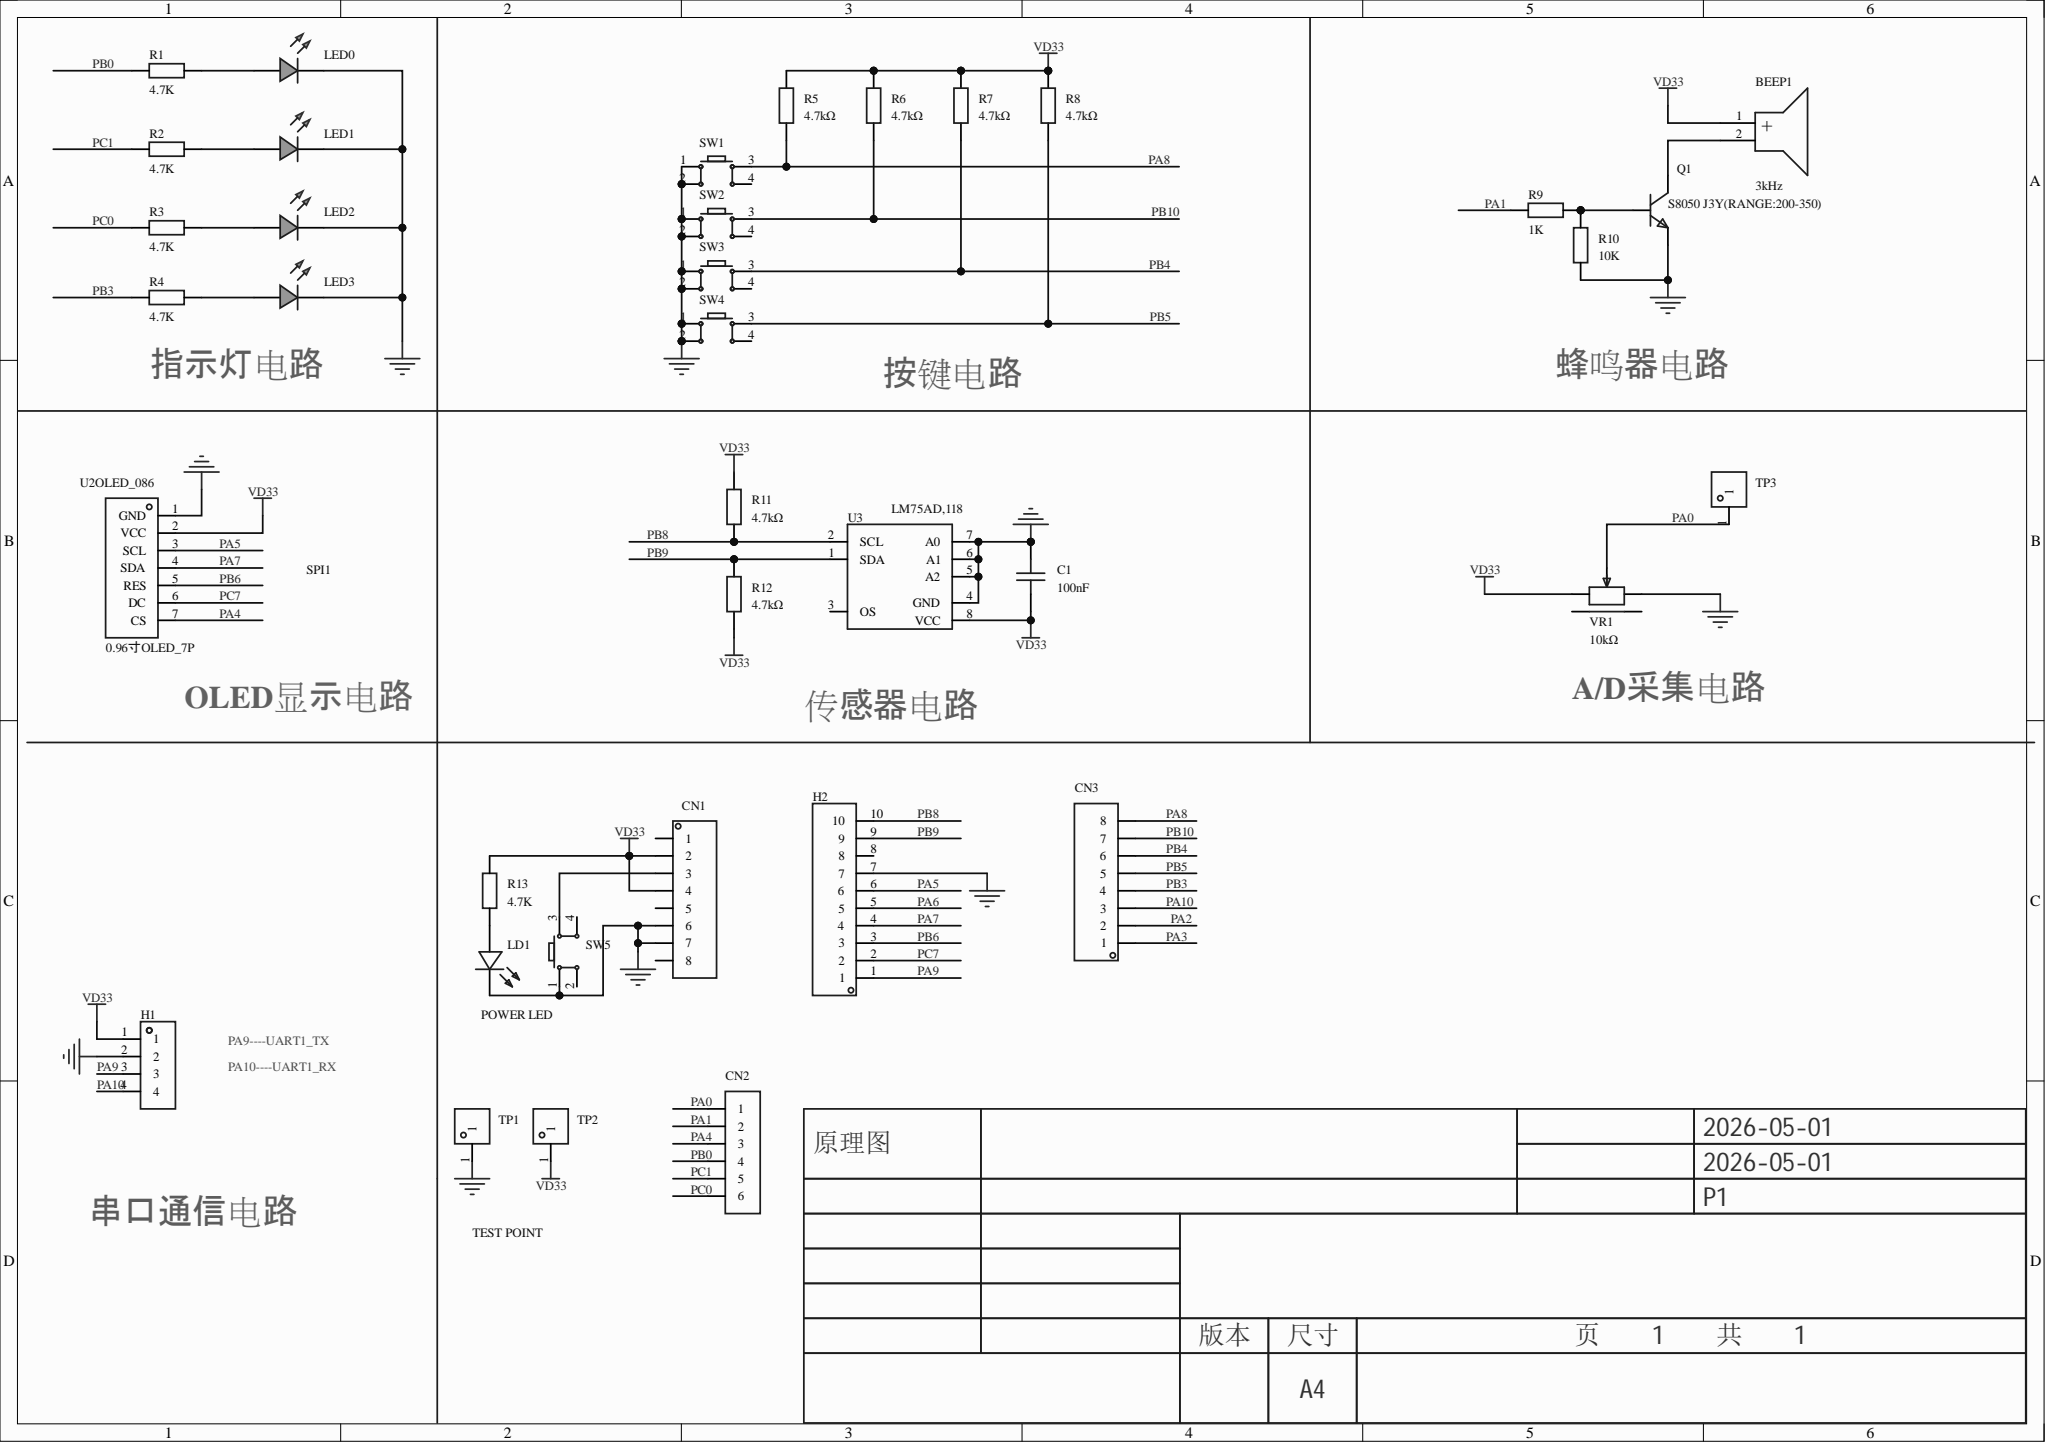Circuit board | Altium Designer | 37 parts | 29 nets
Bill of materials:
Comment,Description,Designator,Footprint,LibRef,Quantity
"3kHz","","BEEP1","BUZ-TH_BD9.0-P5.00-D0.6-FD","HNB09A03","1"
"100nF","","C1","C0805","CC0805KRX7R9BB104","1"
"","","CN1, CN3","HDR-TH_8P-P2.54-V-M","HDR-M_2.54_1x8P","2"
"","","CN2","HDR-TH_6P-P2.54-V-M-1","HDR-M_2.54_1x6P","1"
"","","H1","HDR-TH_4P-P2.54-V-F","HDR-F_2.54_1x4P","1"
"","","H2","HDR-TH_10P-P2.54-V-M-1","HDR-M_2.54_1x10P","1"
"NCD0805R1","","LD1","LED0805-RD","NCD0805R1","1"
"","","LED0, LED1, LED2, LED3","LED_0805","LED_0805-G","4"
"S8050 J3Y(RANGE:200-350)","","Q1","SOT-23-3_L3.0-W1.7-P0.95-LS2.9-BR","S8050 J3Y(RANGE:200-350)","1"
"4.7K","","R1, R2, R3, R4","R0805","Res_0805","4"
"4.7kΩ","","R5, R6, R7, R8, R11, R12","R0805","0805W8F4701T5E","6"
"1K","","R9","R0603","Res_0603","1"
"10K","","R10","R0603","Res_0603","1"
"4.7K","","R13","R0603","Res_0603","1"
"","","SW1, SW2, SW3, SW4, SW5","Key_SMD_4.2x3.2x2.5","Key_SMD_4.2x3.2x2.5","5"
"TP-红色测试点","","TP1, TP2, TP3","TESTPOINT-TH_BD3.2","TP-红色测试点","3"
"0.96寸OLED_7P","","U2OLED_086","OLED-TH_HS96L01W4S03","HS96L01W4S03","1"
"LM75AD,118","","U3","SOIC-8_L5.0-W4.0-P1.27-LS6.0-BL","LM75AD,118","1"
"10kΩ","","VR1","RES-ADJ-TH_RK09K1130AJ3","RK09K1130AJ3","1"
Netlist (Protel format):
[
BEEP1
BUZ-TH_BD9.0-P5.00-D0.6-FD
3kHz



]
[
C1
C0805
100nF



]
[
CN1
HDR-TH_8P-P2.54-V-M




]
[
CN2
HDR-TH_6P-P2.54-V-M-1




]
[
CN3
HDR-TH_8P-P2.54-V-M




]
[
H1
HDR-TH_4P-P2.54-V-F




]
[
H2
HDR-TH_10P-P2.54-V-M-1




]
[
LD1
LED0805-RD
NCD0805R1



]
[
LED0
LED_0805




]
[
LED1
LED_0805




]
[
LED2
LED_0805




]
[
LED3
LED_0805




]
[
Q1
SOT-23-3_L3.0-W1.7-P0.95-LS2.9-BR
S8050 J3Y(RANGE:200-350)



]
[
R1
R0805
4.7K



]
[
R2
R0805
4.7K



]
[
R3
R0805
4.7K



]
[
R4
R0805
4.7K



]
[
R5
R0805
4.7kΩ



]
[
R6
R0805
4.7kΩ



]
[
R7
R0805
4.7kΩ



]
[
R8
R0805
4.7kΩ



]
[
R9
R0603
1K



]
[
R10
R0603
10K



]
[
R11
R0805
4.7kΩ



]
[
R12
R0805
4.7kΩ



]
[
R13
R0603
4.7K



]
[
SW1
Key_SMD_4.2x3.2x2.5




]
[
SW2
Key_SMD_4.2x3.2x2.5




]
[
SW3
Key_SMD_4.2x3.2x2.5




]
[
SW4
Key_SMD_4.2x3.2x2.5




]
[
SW5
Key_SMD_4.2x3.2x2.5




]
[
TP1
TESTPOINT-TH_BD3.2
TP-红色测试点



]
[
TP2
TESTPOINT-TH_BD3.2
TP-红色测试点



]
[
TP3
TESTPOINT-TH_BD3.2
TP-红色测试点



]
[
U2OLED_086
OLED-TH_HS96L01W4S03
0.96寸OLED_7P



]
[
U3
SOIC-8_L5.0-W4.0-P1.27-LS6.0-BL
LM75AD,118



]
[
VR1
RES-ADJ-TH_RK09K1130AJ3
10kΩ



]
(
VD33
BEEP1-1
C1-1
CN1-2
CN1-4
H1-1
R5-2
R6-2
R7-2
R8-2
R11-2
R12-1
R13-2
TP2-1
U2OLED_086-2
U3-8
VR1-3
)
(
PC7
H2-2
U2OLED_086-6
)
(
PC1
CN2-5
R2-1
)
(
PC0
CN2-6
R3-1
)
(
PB10
CN3-7
R6-1
SW2-3
)
(
PB9
H2-9
R12-2
U3-1
)
(
PB8
H2-10
R11-1
U3-2
)
(
PB6
H2-3
U2OLED_086-5
)
(
PB5
CN3-5
R8-1
SW4-3
)
(
PB4
CN3-6
R7-1
SW3-3
)
(
PB3
CN3-4
R4-1
)
(
PB0
CN2-4
R1-1
)
(
PA10
CN3-3
H1-4
)
(
PA9
H1-3
H2-1
)
(
PA8
CN3-8
R5-1
SW1-3
)
(
PA7
H2-4
U2OLED_086-4
)
(
PA5
H2-6
U2OLED_086-3
)
(
PA4
CN2-3
U2OLED_086-7
)
(
PA1
CN2-2
R9-2
)
(
PA0
CN2-1
TP3-1
VR1-2
)
(
NetQ1_1
Q1-1
R9-1
R10-2
)
(
NetLED3_2
LED3-2
R4-2
)
(
NetLED2_2
LED2-2
R3-2
)
(
NetLED1_2
LED1-2
R2-2
)
(
NetLED0_2
LED0-2
R1-2
)
(
NetLD1_2
LD1-2
R13-1
)
(
NetCN1_3
CN1-3
SW5-3
)
(
NetBEEP1_2
BEEP1-2
Q1-3
)
(
GND
C1-2
CN1-6
CN1-7
H1-2
H2-7
LD1-1
LED0-1
LED1-1
LED2-1
LED3-1
Q1-2
R10-1
SW1-1
SW1-2
SW2-1
SW2-2
SW3-1
SW3-2
SW4-1
SW4-2
SW5-1
TP1-1
U2OLED_086-1
U3-4
U3-5
U3-6
U3-7
VR1-1
)